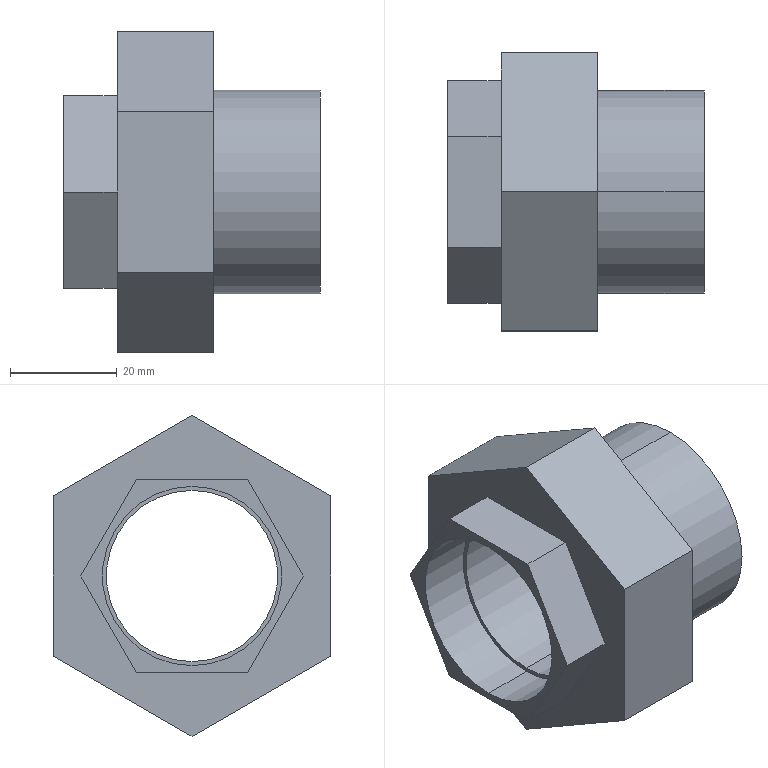Part | SolidWorks | features ICE 2, ExtruThin 1 | 1 solid | 23 faces | box 48 x 51.962 x 60 mm | volume 36619 mm3 | plane 17 | cylinder 6 | commonest cylinder face diameters 32 x2 33.5 x2 38 x2
STEP:
#1=CARTESIAN_POINT('',(-28.,0.,-16.75));
#2=VERTEX_POINT('',#1);
#3=CARTESIAN_POINT('',(-28.,0.,16.75));
#4=VERTEX_POINT('',#3);
#5=CARTESIAN_POINT('',(-28.,0.,0.));
#6=DIRECTION('',(-1.,0.,0.));
#7=DIRECTION('',(0.,0.,1.));
#8=AXIS2_PLACEMENT_3D('',#5,#6,#7);
#9=CIRCLE('',#8,16.75);
#10=EDGE_CURVE('',#2,#4,#9,.T.);
#11=ORIENTED_EDGE('',*,*,#10,.T.);
#12=CARTESIAN_POINT('',(-18.,0.,16.75));
#13=VERTEX_POINT('',#12);
#14=CARTESIAN_POINT('',(-28.,0.,16.75));
#15=DIRECTION('',(1.,0.,0.));
#16=VECTOR('',#15,1000.);
#17=LINE('',#14,#16);
#18=EDGE_CURVE('',#4,#13,#17,.T.);
#19=ORIENTED_EDGE('',*,*,#18,.T.);
#20=CARTESIAN_POINT('',(-18.,0.,-16.75));
#21=VERTEX_POINT('',#20);
#22=CARTESIAN_POINT('',(-18.,0.,0.));
#23=DIRECTION('',(1.,0.,0.));
#24=DIRECTION('',(0.,0.,1.));
#25=AXIS2_PLACEMENT_3D('',#22,#23,#24);
#26=CIRCLE('',#25,16.75);
#27=EDGE_CURVE('',#13,#21,#26,.T.);
#28=ORIENTED_EDGE('',*,*,#27,.T.);
#29=CARTESIAN_POINT('',(-28.,0.,-16.75));
#30=DIRECTION('',(1.,0.,0.));
#31=VECTOR('',#30,1000.);
#32=LINE('',#29,#31);
#33=EDGE_CURVE('',#2,#21,#32,.T.);
#34=ORIENTED_EDGE('',*,*,#33,.F.);
#35=EDGE_LOOP('',(#11,#19,#28,#34));
#36=FACE_OUTER_BOUND('',#35,.T.);
#37=CARTESIAN_POINT('',(-28.,0.,0.));
#38=DIRECTION('',(1.,0.,0.));
#39=DIRECTION('',(0.,0.,-1.));
#40=AXIS2_PLACEMENT_3D('',#37,#38,#39);
#41=CYLINDRICAL_SURFACE('',#40,16.75);
#42=ADVANCED_FACE('',(#36),#41,.F.);
#43=CARTESIAN_POINT('',(20.,0.,16.));
#44=VERTEX_POINT('',#43);
#45=CARTESIAN_POINT('',(20.,0.,-16.));
#46=VERTEX_POINT('',#45);
#47=CARTESIAN_POINT('',(20.,0.,0.));
#48=DIRECTION('',(1.,0.,0.));
#49=DIRECTION('',(0.,0.,-1.));
#50=AXIS2_PLACEMENT_3D('',#47,#48,#49);
#51=CIRCLE('',#50,16.);
#52=EDGE_CURVE('',#44,#46,#51,.T.);
#53=ORIENTED_EDGE('',*,*,#52,.T.);
#54=CARTESIAN_POINT('',(-18.,0.,-16.));
#55=VERTEX_POINT('',#54);
#56=CARTESIAN_POINT('',(20.,0.,-16.));
#57=DIRECTION('',(-1.,0.,0.));
#58=VECTOR('',#57,1000.);
#59=LINE('',#56,#58);
#60=EDGE_CURVE('',#46,#55,#59,.T.);
#61=ORIENTED_EDGE('',*,*,#60,.T.);
#62=CARTESIAN_POINT('',(-18.,0.,16.));
#63=VERTEX_POINT('',#62);
#64=CARTESIAN_POINT('',(-18.,0.,0.));
#65=DIRECTION('',(-1.,0.,0.));
#66=DIRECTION('',(0.,0.,1.));
#67=AXIS2_PLACEMENT_3D('',#64,#65,#66);
#68=CIRCLE('',#67,16.);
#69=EDGE_CURVE('',#55,#63,#68,.T.);
#70=ORIENTED_EDGE('',*,*,#69,.T.);
#71=CARTESIAN_POINT('',(20.,0.,16.));
#72=DIRECTION('',(-1.,0.,0.));
#73=VECTOR('',#72,1000.);
#74=LINE('',#71,#73);
#75=EDGE_CURVE('',#44,#63,#74,.T.);
#76=ORIENTED_EDGE('',*,*,#75,.F.);
#77=EDGE_LOOP('',(#53,#61,#70,#76));
#78=FACE_OUTER_BOUND('',#77,.T.);
#79=CARTESIAN_POINT('',(20.,0.,0.));
#80=DIRECTION('',(-1.,0.,0.));
#81=DIRECTION('',(0.,0.,1.));
#82=AXIS2_PLACEMENT_3D('',#79,#80,#81);
#83=CYLINDRICAL_SURFACE('',#82,16.);
#84=ADVANCED_FACE('',(#78),#83,.F.);
#85=CARTESIAN_POINT('',(20.,0.,-19.));
#86=VERTEX_POINT('',#85);
#87=CARTESIAN_POINT('',(20.,0.,19.));
#88=VERTEX_POINT('',#87);
#89=CARTESIAN_POINT('',(20.,0.,0.));
#90=DIRECTION('',(1.,0.,0.));
#91=DIRECTION('',(0.,0.,-1.));
#92=AXIS2_PLACEMENT_3D('',#89,#90,#91);
#93=CIRCLE('',#92,19.);
#94=EDGE_CURVE('',#86,#88,#93,.T.);
#95=ORIENTED_EDGE('',*,*,#94,.F.);
#96=CARTESIAN_POINT('',(0.,0.,-19.));
#97=VERTEX_POINT('',#96);
#98=CARTESIAN_POINT('',(20.,0.,-19.));
#99=DIRECTION('',(-1.,0.,0.));
#100=VECTOR('',#99,1000.);
#101=LINE('',#98,#100);
#102=EDGE_CURVE('',#86,#97,#101,.T.);
#103=ORIENTED_EDGE('',*,*,#102,.T.);
#104=CARTESIAN_POINT('',(0.,0.,19.));
#105=VERTEX_POINT('',#104);
#106=CARTESIAN_POINT('',(0.,0.,0.));
#107=DIRECTION('',(-1.,0.,0.));
#108=DIRECTION('',(0.,0.,1.));
#109=AXIS2_PLACEMENT_3D('',#106,#107,#108);
#110=CIRCLE('',#109,19.);
#111=EDGE_CURVE('',#105,#97,#110,.T.);
#112=ORIENTED_EDGE('',*,*,#111,.F.);
#113=CARTESIAN_POINT('',(20.,0.,19.));
#114=DIRECTION('',(-1.,0.,0.));
#115=VECTOR('',#114,1000.);
#116=LINE('',#113,#115);
#117=EDGE_CURVE('',#88,#105,#116,.T.);
#118=ORIENTED_EDGE('',*,*,#117,.F.);
#119=EDGE_LOOP('',(#95,#103,#112,#118));
#120=FACE_OUTER_BOUND('',#119,.T.);
#121=CARTESIAN_POINT('',(20.,0.,0.));
#122=DIRECTION('',(-1.,0.,0.));
#123=DIRECTION('',(0.,0.,1.));
#124=AXIS2_PLACEMENT_3D('',#121,#122,#123);
#125=CYLINDRICAL_SURFACE('',#124,19.);
#126=ADVANCED_FACE('',(#120),#125,.T.);
#127=CARTESIAN_POINT('',(-18.,-25.981,15.));
#128=VERTEX_POINT('',#127);
#129=CARTESIAN_POINT('',(-18.,0.,30.));
#130=VERTEX_POINT('',#129);
#131=CARTESIAN_POINT('',(-18.,-25.981,15.));
#132=DIRECTION('',(0.,0.866,0.5));
#133=VECTOR('',#132,1000.);
#134=LINE('',#131,#133);
#135=EDGE_CURVE('',#128,#130,#134,.T.);
#136=ORIENTED_EDGE('',*,*,#135,.T.);
#137=CARTESIAN_POINT('',(-18.,25.981,15.));
#138=VERTEX_POINT('',#137);
#139=CARTESIAN_POINT('',(-18.,0.,30.));
#140=DIRECTION('',(0.,0.866,-0.5));
#141=VECTOR('',#140,1000.);
#142=LINE('',#139,#141);
#143=EDGE_CURVE('',#130,#138,#142,.T.);
#144=ORIENTED_EDGE('',*,*,#143,.T.);
#145=CARTESIAN_POINT('',(-18.,25.981,-15.));
#146=VERTEX_POINT('',#145);
#147=CARTESIAN_POINT('',(-18.,25.981,15.));
#148=DIRECTION('',(0.,0.,-1.));
#149=VECTOR('',#148,1000.);
#150=LINE('',#147,#149);
#151=EDGE_CURVE('',#138,#146,#150,.T.);
#152=ORIENTED_EDGE('',*,*,#151,.T.);
#153=CARTESIAN_POINT('',(-18.,0.,-30.));
#154=VERTEX_POINT('',#153);
#155=CARTESIAN_POINT('',(-18.,25.981,-15.));
#156=DIRECTION('',(0.,-0.866,-0.5));
#157=VECTOR('',#156,1000.);
#158=LINE('',#155,#157);
#159=EDGE_CURVE('',#146,#154,#158,.T.);
#160=ORIENTED_EDGE('',*,*,#159,.T.);
#161=CARTESIAN_POINT('',(-18.,-25.981,-15.));
#162=VERTEX_POINT('',#161);
#163=CARTESIAN_POINT('',(-18.,0.,-30.));
#164=DIRECTION('',(0.,-0.866,0.5));
#165=VECTOR('',#164,1000.);
#166=LINE('',#163,#165);
#167=EDGE_CURVE('',#154,#162,#166,.T.);
#168=ORIENTED_EDGE('',*,*,#167,.T.);
#169=CARTESIAN_POINT('',(-18.,-25.981,-15.));
#170=DIRECTION('',(0.,0.,1.));
#171=VECTOR('',#170,1000.);
#172=LINE('',#169,#171);
#173=EDGE_CURVE('',#162,#128,#172,.T.);
#174=ORIENTED_EDGE('',*,*,#173,.T.);
#175=EDGE_LOOP('',(#136,#144,#152,#160,#168,#174));
#176=FACE_OUTER_BOUND('',#175,.T.);
#177=CARTESIAN_POINT('',(-18.,20.785,0.));
#178=VERTEX_POINT('',#177);
#179=CARTESIAN_POINT('',(-18.,10.392,-18.));
#180=VERTEX_POINT('',#179);
#181=CARTESIAN_POINT('',(-18.,20.785,0.));
#182=DIRECTION('',(0.,-0.5,-0.866));
#183=VECTOR('',#182,1000.);
#184=LINE('',#181,#183);
#185=EDGE_CURVE('',#178,#180,#184,.T.);
#186=ORIENTED_EDGE('',*,*,#185,.F.);
#187=CARTESIAN_POINT('',(-18.,10.392,18.));
#188=VERTEX_POINT('',#187);
#189=CARTESIAN_POINT('',(-18.,10.392,18.));
#190=DIRECTION('',(0.,0.5,-0.866));
#191=VECTOR('',#190,1000.);
#192=LINE('',#189,#191);
#193=EDGE_CURVE('',#188,#178,#192,.T.);
#194=ORIENTED_EDGE('',*,*,#193,.F.);
#195=CARTESIAN_POINT('',(-18.,-10.392,18.));
#196=VERTEX_POINT('',#195);
#197=CARTESIAN_POINT('',(-18.,-10.392,18.));
#198=DIRECTION('',(0.,1.,0.));
#199=VECTOR('',#198,1000.);
#200=LINE('',#197,#199);
#201=EDGE_CURVE('',#196,#188,#200,.T.);
#202=ORIENTED_EDGE('',*,*,#201,.F.);
#203=CARTESIAN_POINT('',(-18.,-20.785,0.));
#204=VERTEX_POINT('',#203);
#205=CARTESIAN_POINT('',(-18.,-20.785,0.));
#206=DIRECTION('',(0.,0.5,0.866));
#207=VECTOR('',#206,1000.);
#208=LINE('',#205,#207);
#209=EDGE_CURVE('',#204,#196,#208,.T.);
#210=ORIENTED_EDGE('',*,*,#209,.F.);
#211=CARTESIAN_POINT('',(-18.,-10.392,-18.));
#212=VERTEX_POINT('',#211);
#213=CARTESIAN_POINT('',(-18.,-10.392,-18.));
#214=DIRECTION('',(0.,-0.5,0.866));
#215=VECTOR('',#214,1000.);
#216=LINE('',#213,#215);
#217=EDGE_CURVE('',#212,#204,#216,.T.);
#218=ORIENTED_EDGE('',*,*,#217,.F.);
#219=CARTESIAN_POINT('',(-18.,10.392,-18.));
#220=DIRECTION('',(0.,-1.,0.));
#221=VECTOR('',#220,1000.);
#222=LINE('',#219,#221);
#223=EDGE_CURVE('',#180,#212,#222,.T.);
#224=ORIENTED_EDGE('',*,*,#223,.F.);
#225=EDGE_LOOP('',(#186,#194,#202,#210,#218,#224));
#226=FACE_BOUND('',#225,.T.);
#227=CARTESIAN_POINT('',(-18.,0.,0.));
#228=DIRECTION('',(-1.,0.,0.));
#229=DIRECTION('',(0.,0.,1.));
#230=AXIS2_PLACEMENT_3D('',#227,#228,#229);
#231=PLANE('',#230);
#232=ADVANCED_FACE('',(#176,#226),#231,.T.);
#233=CARTESIAN_POINT('',(20.,0.,0.));
#234=DIRECTION('',(1.,0.,0.));
#235=DIRECTION('',(0.,0.,-1.));
#236=AXIS2_PLACEMENT_3D('',#233,#234,#235);
#237=CIRCLE('',#236,19.);
#238=EDGE_CURVE('',#88,#86,#237,.T.);
#239=ORIENTED_EDGE('',*,*,#238,.T.);
#240=ORIENTED_EDGE('',*,*,#94,.T.);
#241=EDGE_LOOP('',(#239,#240));
#242=FACE_OUTER_BOUND('',#241,.T.);
#243=ORIENTED_EDGE('',*,*,#52,.F.);
#244=CARTESIAN_POINT('',(20.,0.,0.));
#245=DIRECTION('',(1.,0.,0.));
#246=DIRECTION('',(0.,0.,-1.));
#247=AXIS2_PLACEMENT_3D('',#244,#245,#246);
#248=CIRCLE('',#247,16.);
#249=EDGE_CURVE('',#46,#44,#248,.T.);
#250=ORIENTED_EDGE('',*,*,#249,.F.);
#251=EDGE_LOOP('',(#243,#250));
#252=FACE_BOUND('',#251,.T.);
#253=CARTESIAN_POINT('',(20.,0.,0.));
#254=DIRECTION('',(1.,0.,0.));
#255=DIRECTION('',(0.,0.,-1.));
#256=AXIS2_PLACEMENT_3D('',#253,#254,#255);
#257=PLANE('',#256);
#258=ADVANCED_FACE('',(#242,#252),#257,.T.);
#259=ORIENTED_EDGE('',*,*,#102,.F.);
#260=ORIENTED_EDGE('',*,*,#238,.F.);
#261=ORIENTED_EDGE('',*,*,#117,.T.);
#262=CARTESIAN_POINT('',(0.,0.,0.));
#263=DIRECTION('',(-1.,0.,0.));
#264=DIRECTION('',(0.,0.,1.));
#265=AXIS2_PLACEMENT_3D('',#262,#263,#264);
#266=CIRCLE('',#265,19.);
#267=EDGE_CURVE('',#97,#105,#266,.T.);
#268=ORIENTED_EDGE('',*,*,#267,.F.);
#269=EDGE_LOOP('',(#259,#260,#261,#268));
#270=FACE_OUTER_BOUND('',#269,.T.);
#271=CARTESIAN_POINT('',(20.,0.,0.));
#272=DIRECTION('',(-1.,0.,0.));
#273=DIRECTION('',(0.,0.,1.));
#274=AXIS2_PLACEMENT_3D('',#271,#272,#273);
#275=CYLINDRICAL_SURFACE('',#274,19.);
#276=ADVANCED_FACE('',(#270),#275,.T.);
#277=ORIENTED_EDGE('',*,*,#60,.F.);
#278=ORIENTED_EDGE('',*,*,#249,.T.);
#279=ORIENTED_EDGE('',*,*,#75,.T.);
#280=CARTESIAN_POINT('',(-18.,0.,0.));
#281=DIRECTION('',(-1.,0.,0.));
#282=DIRECTION('',(0.,0.,1.));
#283=AXIS2_PLACEMENT_3D('',#280,#281,#282);
#284=CIRCLE('',#283,16.);
#285=EDGE_CURVE('',#63,#55,#284,.T.);
#286=ORIENTED_EDGE('',*,*,#285,.T.);
#287=EDGE_LOOP('',(#277,#278,#279,#286));
#288=FACE_OUTER_BOUND('',#287,.T.);
#289=CARTESIAN_POINT('',(20.,0.,0.));
#290=DIRECTION('',(-1.,0.,0.));
#291=DIRECTION('',(0.,0.,1.));
#292=AXIS2_PLACEMENT_3D('',#289,#290,#291);
#293=CYLINDRICAL_SURFACE('',#292,16.);
#294=ADVANCED_FACE('',(#288),#293,.F.);
#295=CARTESIAN_POINT('',(0.,-25.981,15.));
#296=VERTEX_POINT('',#295);
#297=CARTESIAN_POINT('',(0.,0.,30.));
#298=VERTEX_POINT('',#297);
#299=CARTESIAN_POINT('',(0.,-25.981,15.));
#300=DIRECTION('',(0.,0.866,0.5));
#301=VECTOR('',#300,1000.);
#302=LINE('',#299,#301);
#303=EDGE_CURVE('',#296,#298,#302,.T.);
#304=ORIENTED_EDGE('',*,*,#303,.F.);
#305=CARTESIAN_POINT('',(0.,-25.981,-15.));
#306=VERTEX_POINT('',#305);
#307=CARTESIAN_POINT('',(0.,-25.981,-15.));
#308=DIRECTION('',(0.,0.,1.));
#309=VECTOR('',#308,1000.);
#310=LINE('',#307,#309);
#311=EDGE_CURVE('',#306,#296,#310,.T.);
#312=ORIENTED_EDGE('',*,*,#311,.F.);
#313=CARTESIAN_POINT('',(0.,0.,-30.));
#314=VERTEX_POINT('',#313);
#315=CARTESIAN_POINT('',(0.,0.,-30.));
#316=DIRECTION('',(0.,-0.866,0.5));
#317=VECTOR('',#316,1000.);
#318=LINE('',#315,#317);
#319=EDGE_CURVE('',#314,#306,#318,.T.);
#320=ORIENTED_EDGE('',*,*,#319,.F.);
#321=CARTESIAN_POINT('',(0.,25.981,-15.));
#322=VERTEX_POINT('',#321);
#323=CARTESIAN_POINT('',(0.,25.981,-15.));
#324=DIRECTION('',(0.,-0.866,-0.5));
#325=VECTOR('',#324,1000.);
#326=LINE('',#323,#325);
#327=EDGE_CURVE('',#322,#314,#326,.T.);
#328=ORIENTED_EDGE('',*,*,#327,.F.);
#329=CARTESIAN_POINT('',(0.,25.981,15.));
#330=VERTEX_POINT('',#329);
#331=CARTESIAN_POINT('',(0.,25.981,15.));
#332=DIRECTION('',(0.,0.,-1.));
#333=VECTOR('',#332,1000.);
#334=LINE('',#331,#333);
#335=EDGE_CURVE('',#330,#322,#334,.T.);
#336=ORIENTED_EDGE('',*,*,#335,.F.);
#337=CARTESIAN_POINT('',(0.,0.,30.));
#338=DIRECTION('',(0.,0.866,-0.5));
#339=VECTOR('',#338,1000.);
#340=LINE('',#337,#339);
#341=EDGE_CURVE('',#298,#330,#340,.T.);
#342=ORIENTED_EDGE('',*,*,#341,.F.);
#343=EDGE_LOOP('',(#304,#312,#320,#328,#336,#342));
#344=FACE_OUTER_BOUND('',#343,.T.);
#345=ORIENTED_EDGE('',*,*,#111,.T.);
#346=ORIENTED_EDGE('',*,*,#267,.T.);
#347=EDGE_LOOP('',(#345,#346));
#348=FACE_BOUND('',#347,.T.);
#349=CARTESIAN_POINT('',(0.,0.,0.));
#350=DIRECTION('',(-1.,0.,0.));
#351=DIRECTION('',(0.,0.,1.));
#352=AXIS2_PLACEMENT_3D('',#349,#350,#351);
#353=PLANE('',#352);
#354=ADVANCED_FACE('',(#344,#348),#353,.F.);
#355=CARTESIAN_POINT('',(-18.,0.,0.));
#356=DIRECTION('',(1.,0.,0.));
#357=DIRECTION('',(0.,0.,1.));
#358=AXIS2_PLACEMENT_3D('',#355,#356,#357);
#359=CIRCLE('',#358,16.75);
#360=EDGE_CURVE('',#21,#13,#359,.T.);
#361=ORIENTED_EDGE('',*,*,#360,.F.);
#362=ORIENTED_EDGE('',*,*,#27,.F.);
#363=EDGE_LOOP('',(#361,#362));
#364=FACE_OUTER_BOUND('',#363,.T.);
#365=ORIENTED_EDGE('',*,*,#285,.F.);
#366=ORIENTED_EDGE('',*,*,#69,.F.);
#367=EDGE_LOOP('',(#365,#366));
#368=FACE_BOUND('',#367,.T.);
#369=CARTESIAN_POINT('',(-18.,0.,0.));
#370=DIRECTION('',(-1.,0.,0.));
#371=DIRECTION('',(0.,0.,1.));
#372=AXIS2_PLACEMENT_3D('',#369,#370,#371);
#373=PLANE('',#372);
#374=ADVANCED_FACE('',(#364,#368),#373,.T.);
#375=ORIENTED_EDGE('',*,*,#303,.T.);
#376=CARTESIAN_POINT('',(-18.,0.,30.));
#377=DIRECTION('',(1.,0.,0.));
#378=VECTOR('',#377,1000.);
#379=LINE('',#376,#378);
#380=EDGE_CURVE('',#130,#298,#379,.T.);
#381=ORIENTED_EDGE('',*,*,#380,.F.);
#382=ORIENTED_EDGE('',*,*,#135,.F.);
#383=CARTESIAN_POINT('',(-18.,-25.981,15.));
#384=DIRECTION('',(1.,0.,0.));
#385=VECTOR('',#384,1000.);
#386=LINE('',#383,#385);
#387=EDGE_CURVE('',#128,#296,#386,.T.);
#388=ORIENTED_EDGE('',*,*,#387,.T.);
#389=EDGE_LOOP('',(#375,#381,#382,#388));
#390=FACE_OUTER_BOUND('',#389,.T.);
#391=CARTESIAN_POINT('',(-18.,-25.981,15.));
#392=DIRECTION('',(0.,0.5,-0.866));
#393=DIRECTION('',(0.,0.866,0.5));
#394=AXIS2_PLACEMENT_3D('',#391,#392,#393);
#395=PLANE('',#394);
#396=ADVANCED_FACE('',(#390),#395,.F.);
#397=ORIENTED_EDGE('',*,*,#341,.T.);
#398=CARTESIAN_POINT('',(-18.,25.981,15.));
#399=DIRECTION('',(1.,0.,0.));
#400=VECTOR('',#399,1000.);
#401=LINE('',#398,#400);
#402=EDGE_CURVE('',#138,#330,#401,.T.);
#403=ORIENTED_EDGE('',*,*,#402,.F.);
#404=ORIENTED_EDGE('',*,*,#143,.F.);
#405=ORIENTED_EDGE('',*,*,#380,.T.);
#406=EDGE_LOOP('',(#397,#403,#404,#405));
#407=FACE_OUTER_BOUND('',#406,.T.);
#408=CARTESIAN_POINT('',(-18.,0.,30.));
#409=DIRECTION('',(0.,-0.5,-0.866));
#410=DIRECTION('',(0.,0.866,-0.5));
#411=AXIS2_PLACEMENT_3D('',#408,#409,#410);
#412=PLANE('',#411);
#413=ADVANCED_FACE('',(#407),#412,.F.);
#414=ORIENTED_EDGE('',*,*,#335,.T.);
#415=CARTESIAN_POINT('',(-18.,25.981,-15.));
#416=DIRECTION('',(1.,0.,0.));
#417=VECTOR('',#416,1000.);
#418=LINE('',#415,#417);
#419=EDGE_CURVE('',#146,#322,#418,.T.);
#420=ORIENTED_EDGE('',*,*,#419,.F.);
#421=ORIENTED_EDGE('',*,*,#151,.F.);
#422=ORIENTED_EDGE('',*,*,#402,.T.);
#423=EDGE_LOOP('',(#414,#420,#421,#422));
#424=FACE_OUTER_BOUND('',#423,.T.);
#425=CARTESIAN_POINT('',(-18.,25.981,15.));
#426=DIRECTION('',(0.,-1.,0.));
#427=DIRECTION('',(0.,0.,-1.));
#428=AXIS2_PLACEMENT_3D('',#425,#426,#427);
#429=PLANE('',#428);
#430=ADVANCED_FACE('',(#424),#429,.F.);
#431=ORIENTED_EDGE('',*,*,#327,.T.);
#432=CARTESIAN_POINT('',(-18.,0.,-30.));
#433=DIRECTION('',(1.,0.,0.));
#434=VECTOR('',#433,1000.);
#435=LINE('',#432,#434);
#436=EDGE_CURVE('',#154,#314,#435,.T.);
#437=ORIENTED_EDGE('',*,*,#436,.F.);
#438=ORIENTED_EDGE('',*,*,#159,.F.);
#439=ORIENTED_EDGE('',*,*,#419,.T.);
#440=EDGE_LOOP('',(#431,#437,#438,#439));
#441=FACE_OUTER_BOUND('',#440,.T.);
#442=CARTESIAN_POINT('',(-18.,25.981,-15.));
#443=DIRECTION('',(0.,-0.5,0.866));
#444=DIRECTION('',(0.,-0.866,-0.5));
#445=AXIS2_PLACEMENT_3D('',#442,#443,#444);
#446=PLANE('',#445);
#447=ADVANCED_FACE('',(#441),#446,.F.);
#448=ORIENTED_EDGE('',*,*,#319,.T.);
#449=CARTESIAN_POINT('',(-18.,-25.981,-15.));
#450=DIRECTION('',(1.,0.,0.));
#451=VECTOR('',#450,1000.);
#452=LINE('',#449,#451);
#453=EDGE_CURVE('',#162,#306,#452,.T.);
#454=ORIENTED_EDGE('',*,*,#453,.F.);
#455=ORIENTED_EDGE('',*,*,#167,.F.);
#456=ORIENTED_EDGE('',*,*,#436,.T.);
#457=EDGE_LOOP('',(#448,#454,#455,#456));
#458=FACE_OUTER_BOUND('',#457,.T.);
#459=CARTESIAN_POINT('',(-18.,0.,-30.));
#460=DIRECTION('',(0.,0.5,0.866));
#461=DIRECTION('',(0.,-0.866,0.5));
#462=AXIS2_PLACEMENT_3D('',#459,#460,#461);
#463=PLANE('',#462);
#464=ADVANCED_FACE('',(#458),#463,.F.);
#465=ORIENTED_EDGE('',*,*,#311,.T.);
#466=ORIENTED_EDGE('',*,*,#387,.F.);
#467=ORIENTED_EDGE('',*,*,#173,.F.);
#468=ORIENTED_EDGE('',*,*,#453,.T.);
#469=EDGE_LOOP('',(#465,#466,#467,#468));
#470=FACE_OUTER_BOUND('',#469,.T.);
#471=CARTESIAN_POINT('',(-18.,-25.981,-15.));
#472=DIRECTION('',(0.,1.,0.));
#473=DIRECTION('',(0.,0.,1.));
#474=AXIS2_PLACEMENT_3D('',#471,#472,#473);
#475=PLANE('',#474);
#476=ADVANCED_FACE('',(#470),#475,.F.);
#477=CARTESIAN_POINT('',(-28.,10.392,18.));
#478=VERTEX_POINT('',#477);
#479=CARTESIAN_POINT('',(-28.,20.785,0.));
#480=VERTEX_POINT('',#479);
#481=CARTESIAN_POINT('',(-28.,10.392,18.));
#482=DIRECTION('',(0.,0.5,-0.866));
#483=VECTOR('',#482,1000.);
#484=LINE('',#481,#483);
#485=EDGE_CURVE('',#478,#480,#484,.T.);
#486=ORIENTED_EDGE('',*,*,#485,.T.);
#487=CARTESIAN_POINT('',(-28.,10.392,-18.));
#488=VERTEX_POINT('',#487);
#489=CARTESIAN_POINT('',(-28.,20.785,0.));
#490=DIRECTION('',(0.,-0.5,-0.866));
#491=VECTOR('',#490,1000.);
#492=LINE('',#489,#491);
#493=EDGE_CURVE('',#480,#488,#492,.T.);
#494=ORIENTED_EDGE('',*,*,#493,.T.);
#495=CARTESIAN_POINT('',(-28.,-10.392,-18.));
#496=VERTEX_POINT('',#495);
#497=CARTESIAN_POINT('',(-28.,10.392,-18.));
#498=DIRECTION('',(0.,-1.,0.));
#499=VECTOR('',#498,1000.);
#500=LINE('',#497,#499);
#501=EDGE_CURVE('',#488,#496,#500,.T.);
#502=ORIENTED_EDGE('',*,*,#501,.T.);
#503=CARTESIAN_POINT('',(-28.,-20.785,0.));
#504=VERTEX_POINT('',#503);
#505=CARTESIAN_POINT('',(-28.,-10.392,-18.));
#506=DIRECTION('',(0.,-0.5,0.866));
#507=VECTOR('',#506,1000.);
#508=LINE('',#505,#507);
#509=EDGE_CURVE('',#496,#504,#508,.T.);
#510=ORIENTED_EDGE('',*,*,#509,.T.);
#511=CARTESIAN_POINT('',(-28.,-10.392,18.));
#512=VERTEX_POINT('',#511);
#513=CARTESIAN_POINT('',(-28.,-20.785,0.));
#514=DIRECTION('',(0.,0.5,0.866));
#515=VECTOR('',#514,1000.);
#516=LINE('',#513,#515);
#517=EDGE_CURVE('',#504,#512,#516,.T.);
#518=ORIENTED_EDGE('',*,*,#517,.T.);
#519=CARTESIAN_POINT('',(-28.,-10.392,18.));
#520=DIRECTION('',(0.,1.,0.));
#521=VECTOR('',#520,1000.);
#522=LINE('',#519,#521);
#523=EDGE_CURVE('',#512,#478,#522,.T.);
#524=ORIENTED_EDGE('',*,*,#523,.T.);
#525=EDGE_LOOP('',(#486,#494,#502,#510,#518,#524));
#526=FACE_OUTER_BOUND('',#525,.T.);
#527=ORIENTED_EDGE('',*,*,#10,.F.);
#528=CARTESIAN_POINT('',(-28.,0.,0.));
#529=DIRECTION('',(-1.,0.,0.));
#530=DIRECTION('',(0.,0.,1.));
#531=AXIS2_PLACEMENT_3D('',#528,#529,#530);
#532=CIRCLE('',#531,16.75);
#533=EDGE_CURVE('',#4,#2,#532,.T.);
#534=ORIENTED_EDGE('',*,*,#533,.F.);
#535=EDGE_LOOP('',(#527,#534));
#536=FACE_BOUND('',#535,.T.);
#537=CARTESIAN_POINT('',(-28.,0.,0.));
#538=DIRECTION('',(-1.,0.,0.));
#539=DIRECTION('',(0.,0.,1.));
#540=AXIS2_PLACEMENT_3D('',#537,#538,#539);
#541=PLANE('',#540);
#542=ADVANCED_FACE('',(#526,#536),#541,.T.);
#543=ORIENTED_EDGE('',*,*,#193,.T.);
#544=CARTESIAN_POINT('',(-28.,20.785,0.));
#545=DIRECTION('',(1.,0.,0.));
#546=VECTOR('',#545,1000.);
#547=LINE('',#544,#546);
#548=EDGE_CURVE('',#480,#178,#547,.T.);
#549=ORIENTED_EDGE('',*,*,#548,.F.);
#550=ORIENTED_EDGE('',*,*,#485,.F.);
#551=CARTESIAN_POINT('',(-28.,10.392,18.));
#552=DIRECTION('',(1.,0.,0.));
#553=VECTOR('',#552,1000.);
#554=LINE('',#551,#553);
#555=EDGE_CURVE('',#478,#188,#554,.T.);
#556=ORIENTED_EDGE('',*,*,#555,.T.);
#557=EDGE_LOOP('',(#543,#549,#550,#556));
#558=FACE_OUTER_BOUND('',#557,.T.);
#559=CARTESIAN_POINT('',(-28.,10.392,18.));
#560=DIRECTION('',(0.,-0.866,-0.5));
#561=DIRECTION('',(0.,0.5,-0.866));
#562=AXIS2_PLACEMENT_3D('',#559,#560,#561);
#563=PLANE('',#562);
#564=ADVANCED_FACE('',(#558),#563,.F.);
#565=ORIENTED_EDGE('',*,*,#185,.T.);
#566=CARTESIAN_POINT('',(-28.,10.392,-18.));
#567=DIRECTION('',(1.,0.,0.));
#568=VECTOR('',#567,1000.);
#569=LINE('',#566,#568);
#570=EDGE_CURVE('',#488,#180,#569,.T.);
#571=ORIENTED_EDGE('',*,*,#570,.F.);
#572=ORIENTED_EDGE('',*,*,#493,.F.);
#573=ORIENTED_EDGE('',*,*,#548,.T.);
#574=EDGE_LOOP('',(#565,#571,#572,#573));
#575=FACE_OUTER_BOUND('',#574,.T.);
#576=CARTESIAN_POINT('',(-28.,20.785,0.));
#577=DIRECTION('',(0.,-0.866,0.5));
#578=DIRECTION('',(0.,-0.5,-0.866));
#579=AXIS2_PLACEMENT_3D('',#576,#577,#578);
#580=PLANE('',#579);
#581=ADVANCED_FACE('',(#575),#580,.F.);
#582=ORIENTED_EDGE('',*,*,#223,.T.);
#583=CARTESIAN_POINT('',(-28.,-10.392,-18.));
#584=DIRECTION('',(1.,0.,0.));
#585=VECTOR('',#584,1000.);
#586=LINE('',#583,#585);
#587=EDGE_CURVE('',#496,#212,#586,.T.);
#588=ORIENTED_EDGE('',*,*,#587,.F.);
#589=ORIENTED_EDGE('',*,*,#501,.F.);
#590=ORIENTED_EDGE('',*,*,#570,.T.);
#591=EDGE_LOOP('',(#582,#588,#589,#590));
#592=FACE_OUTER_BOUND('',#591,.T.);
#593=CARTESIAN_POINT('',(-28.,10.392,-18.));
#594=DIRECTION('',(0.,0.,1.));
#595=DIRECTION('',(1.,0.,0.));
#596=AXIS2_PLACEMENT_3D('',#593,#594,#595);
#597=PLANE('',#596);
#598=ADVANCED_FACE('',(#592),#597,.F.);
#599=ORIENTED_EDGE('',*,*,#217,.T.);
#600=CARTESIAN_POINT('',(-28.,-20.785,0.));
#601=DIRECTION('',(1.,0.,0.));
#602=VECTOR('',#601,1000.);
#603=LINE('',#600,#602);
#604=EDGE_CURVE('',#504,#204,#603,.T.);
#605=ORIENTED_EDGE('',*,*,#604,.F.);
#606=ORIENTED_EDGE('',*,*,#509,.F.);
#607=ORIENTED_EDGE('',*,*,#587,.T.);
#608=EDGE_LOOP('',(#599,#605,#606,#607));
#609=FACE_OUTER_BOUND('',#608,.T.);
#610=CARTESIAN_POINT('',(-28.,-10.392,-18.));
#611=DIRECTION('',(0.,0.866,0.5));
#612=DIRECTION('',(0.,-0.5,0.866));
#613=AXIS2_PLACEMENT_3D('',#610,#611,#612);
#614=PLANE('',#613);
#615=ADVANCED_FACE('',(#609),#614,.F.);
#616=ORIENTED_EDGE('',*,*,#209,.T.);
#617=CARTESIAN_POINT('',(-28.,-10.392,18.));
#618=DIRECTION('',(1.,0.,0.));
#619=VECTOR('',#618,1000.);
#620=LINE('',#617,#619);
#621=EDGE_CURVE('',#512,#196,#620,.T.);
#622=ORIENTED_EDGE('',*,*,#621,.F.);
#623=ORIENTED_EDGE('',*,*,#517,.F.);
#624=ORIENTED_EDGE('',*,*,#604,.T.);
#625=EDGE_LOOP('',(#616,#622,#623,#624));
#626=FACE_OUTER_BOUND('',#625,.T.);
#627=CARTESIAN_POINT('',(-28.,-20.785,0.));
#628=DIRECTION('',(0.,0.866,-0.5));
#629=DIRECTION('',(0.,0.5,0.866));
#630=AXIS2_PLACEMENT_3D('',#627,#628,#629);
#631=PLANE('',#630);
#632=ADVANCED_FACE('',(#626),#631,.F.);
#633=ORIENTED_EDGE('',*,*,#201,.T.);
#634=ORIENTED_EDGE('',*,*,#555,.F.);
#635=ORIENTED_EDGE('',*,*,#523,.F.);
#636=ORIENTED_EDGE('',*,*,#621,.T.);
#637=EDGE_LOOP('',(#633,#634,#635,#636));
#638=FACE_OUTER_BOUND('',#637,.T.);
#639=CARTESIAN_POINT('',(-28.,-10.392,18.));
#640=DIRECTION('',(0.,0.,-1.));
#641=DIRECTION('',(0.,1.,0.));
#642=AXIS2_PLACEMENT_3D('',#639,#640,#641);
#643=PLANE('',#642);
#644=ADVANCED_FACE('',(#638),#643,.F.);
#645=ORIENTED_EDGE('',*,*,#18,.F.);
#646=ORIENTED_EDGE('',*,*,#533,.T.);
#647=ORIENTED_EDGE('',*,*,#33,.T.);
#648=ORIENTED_EDGE('',*,*,#360,.T.);
#649=EDGE_LOOP('',(#645,#646,#647,#648));
#650=FACE_OUTER_BOUND('',#649,.T.);
#651=CARTESIAN_POINT('',(-28.,0.,0.));
#652=DIRECTION('',(1.,0.,0.));
#653=DIRECTION('',(0.,0.,-1.));
#654=AXIS2_PLACEMENT_3D('',#651,#652,#653);
#655=CYLINDRICAL_SURFACE('',#654,16.75);
#656=ADVANCED_FACE('',(#650),#655,.F.);
#657=CLOSED_SHELL('',(#42,#84,#126,#232,#258,#276,#294,#354,#374,#396,#413,#430,#447,#464,#476,#542,#564,#581,#598,#615,#632,#644,#656));
#658=MANIFOLD_SOLID_BREP('',#657);
#659=CARTESIAN_POINT('',(0.,0.,0.));
#660=DIRECTION('',(0.,0.,1.));
#661=DIRECTION('',(1.,0.,0.));
#662=AXIS2_PLACEMENT_3D('',#659,#660,#661);
#663=(LENGTH_UNIT()NAMED_UNIT(*)SI_UNIT(.MILLI.,.METRE.));
#664=UNCERTAINTY_MEASURE_WITH_UNIT(LENGTH_MEASURE(0.00001),#663,'','');
#665=(NAMED_UNIT(*)PLANE_ANGLE_UNIT()SI_UNIT($,.RADIAN.));
#666=(NAMED_UNIT(*)SI_UNIT($,.STERADIAN.)SOLID_ANGLE_UNIT());
#667=(GEOMETRIC_REPRESENTATION_CONTEXT(3)GLOBAL_UNCERTAINTY_ASSIGNED_CONTEXT((#664))GLOBAL_UNIT_ASSIGNED_CONTEXT((#663,#665,#666))REPRESENTATION_CONTEXT('',''));
#668=ADVANCED_BREP_SHAPE_REPRESENTATION('',(#658,#662),#667);